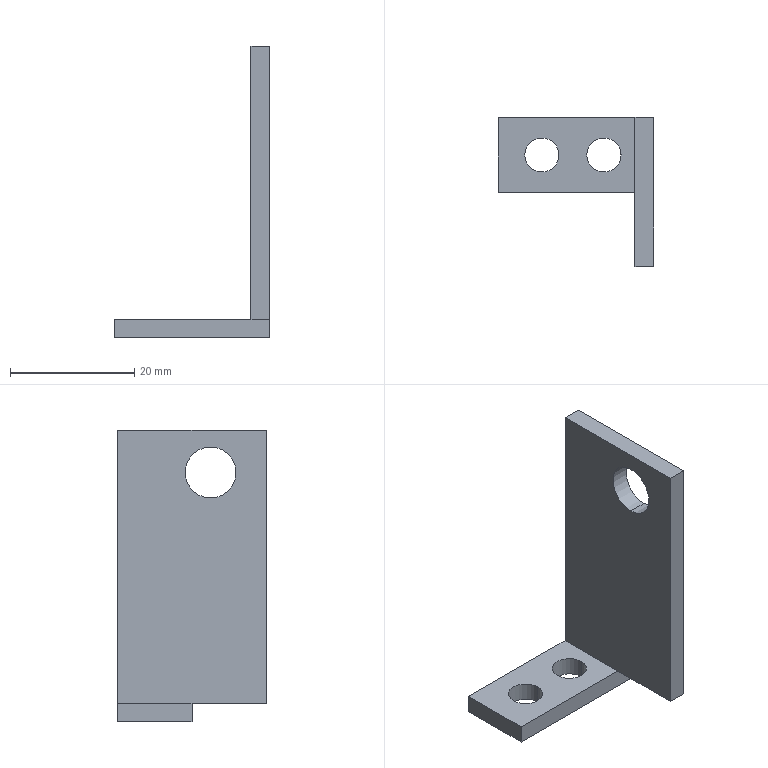Part | 1 solid | 16 faces | box 25 x 24 x 47 mm | volume 3767 mm3 | plane 10 | cylinder 6 | commonest cylinder face diameters 5.5 x4 8.2 x2
STEP:
#1=CARTESIAN_POINT('',(0.,0.,0.));
#2=DIRECTION('',(0.,0.,1.));
#3=DIRECTION('',(1.,0.,0.));
#4=AXIS2_PLACEMENT_3D('',#1,#2,#3);
#5=CARTESIAN_POINT('',(-283.573,419.5,-194.274));
#6=VERTEX_POINT('',#5);
#7=CARTESIAN_POINT('',(-283.573,419.5,-202.474));
#8=VERTEX_POINT('',#7);
#9=CARTESIAN_POINT('',(-283.573,419.5,-198.374));
#10=DIRECTION('',(-1.,0.,0.));
#11=DIRECTION('',(0.,0.,-1.));
#12=AXIS2_PLACEMENT_3D('',#9,#10,#11);
#13=CIRCLE('',#12,4.1);
#14=CARTESIAN_POINT('',(-291.041,419.5,-198.374));
#15=DIRECTION('',(-1.,0.,0.));
#16=DIRECTION('',(0.,-1.,0.));
#17=AXIS2_PLACEMENT_3D('',#14,#15,#16);
#18=CYLINDRICAL_SURFACE('',#17,4.1);
#19=CARTESIAN_POINT('',(-1.571,-7.468));
#20=DIRECTION('',(1.,0.));
#21=VECTOR('',#20,1.);
#22=LINE('',#19,#21);
#23=(GEOMETRIC_REPRESENTATION_CONTEXT(2)PARAMETRIC_REPRESENTATION_CONTEXT()REPRESENTATION_CONTEXT('',''));
#24=DEFINITIONAL_REPRESENTATION('',(#22),#23);
#25=PCURVE('',#18,#24);
#26=CARTESIAN_POINT('',(-283.573,428.525,-194.374));
#27=DIRECTION('',(1.,0.,0.));
#28=DIRECTION('',(0.,-1.,0.));
#29=AXIS2_PLACEMENT_3D('',#26,#27,#28);
#30=PLANE('',#29);
#31=CARTESIAN_POINT('',(9.025,8.1));
#32=CARTESIAN_POINT('',(16.126,8.1));
#33=CARTESIAN_POINT('',(12.576,1.95));
#34=CARTESIAN_POINT('',(9.025,-4.2));
#35=CARTESIAN_POINT('',(5.474,1.95));
#36=CARTESIAN_POINT('',(1.924,8.1));
#37=CARTESIAN_POINT('',(9.025,8.1));
#38=(BOUNDED_CURVE()B_SPLINE_CURVE(2,(#31,#32,#33,#34,#35,#36,#37),.UNSPECIFIED.,.T.,.F.)B_SPLINE_CURVE_WITH_KNOTS((1,2,2,2,2,1),(-2.094,0.,2.094,4.189,6.283,8.378),.UNSPECIFIED.)CURVE()GEOMETRIC_REPRESENTATION_ITEM()RATIONAL_B_SPLINE_CURVE((1.,0.5,1.,0.5,1.,0.5,1.))REPRESENTATION_ITEM(''));
#39=(GEOMETRIC_REPRESENTATION_CONTEXT(2)PARAMETRIC_REPRESENTATION_CONTEXT()REPRESENTATION_CONTEXT('',''));
#40=DEFINITIONAL_REPRESENTATION('',(#38),#39);
#41=PCURVE('',#30,#40);
#42=SURFACE_CURVE('',#13,(#25,#41),.PCURVE_S1.);
#43=EDGE_CURVE('',#6,#8,#42,.T.);
#44=ORIENTED_EDGE('',*,*,#43,.T.);
#45=CARTESIAN_POINT('',(-286.573,419.5,-202.474));
#46=VERTEX_POINT('',#45);
#47=CARTESIAN_POINT('',(-283.573,419.5,-202.474));
#48=DIRECTION('',(-1.,0.,0.));
#49=VECTOR('',#48,1.);
#50=LINE('',#47,#49);
#51=CARTESIAN_POINT('',(4.712,-7.468));
#52=DIRECTION('',(0.,1.));
#53=VECTOR('',#52,1.);
#54=LINE('',#51,#53);
#55=(GEOMETRIC_REPRESENTATION_CONTEXT(2)PARAMETRIC_REPRESENTATION_CONTEXT()REPRESENTATION_CONTEXT('',''));
#56=DEFINITIONAL_REPRESENTATION('',(#54),#55);
#57=PCURVE('',#18,#56);
#58=CARTESIAN_POINT('',(-291.041,419.5,-198.374));
#59=DIRECTION('',(-1.,0.,0.));
#60=DIRECTION('',(0.,1.,0.));
#61=AXIS2_PLACEMENT_3D('',#58,#59,#60);
#62=CYLINDRICAL_SURFACE('',#61,4.1);
#63=CARTESIAN_POINT('',(1.571,-7.468));
#64=DIRECTION('',(0.,1.));
#65=VECTOR('',#64,1.);
#66=LINE('',#63,#65);
#67=(GEOMETRIC_REPRESENTATION_CONTEXT(2)PARAMETRIC_REPRESENTATION_CONTEXT()REPRESENTATION_CONTEXT('',''));
#68=DEFINITIONAL_REPRESENTATION('',(#66),#67);
#69=PCURVE('',#62,#68);
#70=SURFACE_CURVE('',#50,(#57,#69),.PCURVE_S1.);
#71=EDGE_CURVE('',#8,#46,#70,.T.);
#72=ORIENTED_EDGE('',*,*,#71,.T.);
#73=CARTESIAN_POINT('',(-286.573,419.5,-194.274));
#74=VERTEX_POINT('',#73);
#75=CARTESIAN_POINT('',(-286.573,419.5,-198.374));
#76=DIRECTION('',(1.,0.,0.));
#77=DIRECTION('',(0.,0.,-1.));
#78=AXIS2_PLACEMENT_3D('',#75,#76,#77);
#79=CIRCLE('',#78,4.1);
#80=CARTESIAN_POINT('',(4.712,-4.468));
#81=DIRECTION('',(-1.,0.));
#82=VECTOR('',#81,1.);
#83=LINE('',#80,#82);
#84=(GEOMETRIC_REPRESENTATION_CONTEXT(2)PARAMETRIC_REPRESENTATION_CONTEXT()REPRESENTATION_CONTEXT('',''));
#85=DEFINITIONAL_REPRESENTATION('',(#83),#84);
#86=PCURVE('',#18,#85);
#87=CARTESIAN_POINT('',(-286.573,428.525,-194.374));
#88=DIRECTION('',(-1.,0.,0.));
#89=DIRECTION('',(0.,1.,0.));
#90=AXIS2_PLACEMENT_3D('',#87,#88,#89);
#91=PLANE('',#90);
#92=CARTESIAN_POINT('',(-9.025,8.1));
#93=CARTESIAN_POINT('',(-1.924,8.1));
#94=CARTESIAN_POINT('',(-5.474,1.95));
#95=CARTESIAN_POINT('',(-9.025,-4.2));
#96=CARTESIAN_POINT('',(-12.576,1.95));
#97=CARTESIAN_POINT('',(-16.126,8.1));
#98=CARTESIAN_POINT('',(-9.025,8.1));
#99=(BOUNDED_CURVE()B_SPLINE_CURVE(2,(#92,#93,#94,#95,#96,#97,#98),.UNSPECIFIED.,.T.,.F.)B_SPLINE_CURVE_WITH_KNOTS((1,2,2,2,2,1),(-2.094,0.,2.094,4.189,6.283,8.378),.UNSPECIFIED.)CURVE()GEOMETRIC_REPRESENTATION_ITEM()RATIONAL_B_SPLINE_CURVE((1.,0.5,1.,0.5,1.,0.5,1.))REPRESENTATION_ITEM(''));
#100=(GEOMETRIC_REPRESENTATION_CONTEXT(2)PARAMETRIC_REPRESENTATION_CONTEXT()REPRESENTATION_CONTEXT('',''));
#101=DEFINITIONAL_REPRESENTATION('',(#99),#100);
#102=PCURVE('',#91,#101);
#103=SURFACE_CURVE('',#79,(#86,#102),.PCURVE_S1.);
#104=EDGE_CURVE('',#46,#74,#103,.T.);
#105=ORIENTED_EDGE('',*,*,#104,.T.);
#106=CARTESIAN_POINT('',(-283.573,419.5,-194.274));
#107=DIRECTION('',(-1.,0.,0.));
#108=VECTOR('',#107,1.);
#109=LINE('',#106,#108);
#110=CARTESIAN_POINT('',(1.571,-7.468));
#111=DIRECTION('',(0.,1.));
#112=VECTOR('',#111,1.);
#113=LINE('',#110,#112);
#114=(GEOMETRIC_REPRESENTATION_CONTEXT(2)PARAMETRIC_REPRESENTATION_CONTEXT()REPRESENTATION_CONTEXT('',''));
#115=DEFINITIONAL_REPRESENTATION('',(#113),#114);
#116=PCURVE('',#18,#115);
#117=CARTESIAN_POINT('',(4.712,-7.468));
#118=DIRECTION('',(0.,1.));
#119=VECTOR('',#118,1.);
#120=LINE('',#117,#119);
#121=(GEOMETRIC_REPRESENTATION_CONTEXT(2)PARAMETRIC_REPRESENTATION_CONTEXT()REPRESENTATION_CONTEXT('',''));
#122=DEFINITIONAL_REPRESENTATION('',(#120),#121);
#123=PCURVE('',#62,#122);
#124=SURFACE_CURVE('',#109,(#116,#123),.PCURVE_S1.);
#125=EDGE_CURVE('',#6,#74,#124,.T.);
#126=ORIENTED_EDGE('',*,*,#125,.F.);
#127=EDGE_LOOP('',(#44,#72,#105,#126));
#128=FACE_BOUND('',#127,.F.);
#129=ADVANCED_FACE('',(#128),#18,.F.);
#130=CARTESIAN_POINT('',(-286.573,410.5,-191.55));
#131=VERTEX_POINT('',#130);
#132=CARTESIAN_POINT('',(-286.573,434.5,-191.55));
#133=VERTEX_POINT('',#132);
#134=CARTESIAN_POINT('',(-286.573,428.525,-191.55));
#135=DIRECTION('',(0.,1.,0.));
#136=VECTOR('',#135,1.);
#137=LINE('',#134,#136);
#138=CARTESIAN_POINT('',(0.,-2.824));
#139=DIRECTION('',(1.,0.));
#140=VECTOR('',#139,1.);
#141=LINE('',#138,#140);
#142=(GEOMETRIC_REPRESENTATION_CONTEXT(2)PARAMETRIC_REPRESENTATION_CONTEXT()REPRESENTATION_CONTEXT('',''));
#143=DEFINITIONAL_REPRESENTATION('',(#141),#142);
#144=PCURVE('',#91,#143);
#145=CARTESIAN_POINT('',(-153.465,586.5,-191.55));
#146=DIRECTION('',(0.,0.,1.));
#147=DIRECTION('',(-1.,0.,0.));
#148=AXIS2_PLACEMENT_3D('',#145,#146,#147);
#149=PLANE('',#148);
#150=CARTESIAN_POINT('',(133.108,157.975));
#151=DIRECTION('',(0.,-1.));
#152=VECTOR('',#151,1.);
#153=LINE('',#150,#152);
#154=(GEOMETRIC_REPRESENTATION_CONTEXT(2)PARAMETRIC_REPRESENTATION_CONTEXT()REPRESENTATION_CONTEXT('',''));
#155=DEFINITIONAL_REPRESENTATION('',(#153),#154);
#156=PCURVE('',#149,#155);
#157=SURFACE_CURVE('',#137,(#144,#156),.PCURVE_S1.);
#158=EDGE_CURVE('',#131,#133,#157,.T.);
#159=ORIENTED_EDGE('',*,*,#158,.T.);
#160=CARTESIAN_POINT('',(-286.573,434.5,-235.55));
#161=VERTEX_POINT('',#160);
#162=CARTESIAN_POINT('',(-286.573,434.5,-194.374));
#163=DIRECTION('',(0.,0.,1.));
#164=VECTOR('',#163,1.);
#165=LINE('',#162,#164);
#166=CARTESIAN_POINT('',(5.975,0.));
#167=DIRECTION('',(0.,-1.));
#168=VECTOR('',#167,1.);
#169=LINE('',#166,#168);
#170=(GEOMETRIC_REPRESENTATION_CONTEXT(2)PARAMETRIC_REPRESENTATION_CONTEXT()REPRESENTATION_CONTEXT('',''));
#171=DEFINITIONAL_REPRESENTATION('',(#169),#170);
#172=PCURVE('',#91,#171);
#173=CARTESIAN_POINT('',(-285.073,434.5,-194.374));
#174=DIRECTION('',(0.,1.,0.));
#175=DIRECTION('',(1.,0.,0.));
#176=AXIS2_PLACEMENT_3D('',#173,#174,#175);
#177=PLANE('',#176);
#178=CARTESIAN_POINT('',(-1.5,0.));
#179=DIRECTION('',(0.,-1.));
#180=VECTOR('',#179,1.);
#181=LINE('',#178,#180);
#182=(GEOMETRIC_REPRESENTATION_CONTEXT(2)PARAMETRIC_REPRESENTATION_CONTEXT()REPRESENTATION_CONTEXT('',''));
#183=DEFINITIONAL_REPRESENTATION('',(#181),#182);
#184=PCURVE('',#177,#183);
#185=SURFACE_CURVE('',#165,(#172,#184),.PCURVE_S1.);
#186=EDGE_CURVE('',#161,#133,#185,.T.);
#187=ORIENTED_EDGE('',*,*,#186,.F.);
#188=CARTESIAN_POINT('',(-286.573,422.5,-235.55));
#189=VERTEX_POINT('',#188);
#190=CARTESIAN_POINT('',(-286.573,428.525,-235.55));
#191=DIRECTION('',(0.,1.,0.));
#192=VECTOR('',#191,1.);
#193=LINE('',#190,#192);
#194=CARTESIAN_POINT('',(0.,41.176));
#195=DIRECTION('',(1.,0.));
#196=VECTOR('',#195,1.);
#197=LINE('',#194,#196);
#198=(GEOMETRIC_REPRESENTATION_CONTEXT(2)PARAMETRIC_REPRESENTATION_CONTEXT()REPRESENTATION_CONTEXT('',''));
#199=DEFINITIONAL_REPRESENTATION('',(#197),#198);
#200=PCURVE('',#91,#199);
#201=CARTESIAN_POINT('',(-153.465,586.5,-235.55));
#202=DIRECTION('',(0.,0.,1.));
#203=DIRECTION('',(-1.,0.,0.));
#204=AXIS2_PLACEMENT_3D('',#201,#202,#203);
#205=PLANE('',#204);
#206=CARTESIAN_POINT('',(133.108,157.975));
#207=DIRECTION('',(0.,-1.));
#208=VECTOR('',#207,1.);
#209=LINE('',#206,#208);
#210=(GEOMETRIC_REPRESENTATION_CONTEXT(2)PARAMETRIC_REPRESENTATION_CONTEXT()REPRESENTATION_CONTEXT('',''));
#211=DEFINITIONAL_REPRESENTATION('',(#209),#210);
#212=PCURVE('',#205,#211);
#213=SURFACE_CURVE('',#193,(#200,#212),.PCURVE_S1.);
#214=EDGE_CURVE('',#189,#161,#213,.T.);
#215=ORIENTED_EDGE('',*,*,#214,.F.);
#216=CARTESIAN_POINT('',(-286.573,410.5,-235.55));
#217=VERTEX_POINT('',#216);
#218=CARTESIAN_POINT('',(-286.573,428.525,-235.55));
#219=DIRECTION('',(0.,1.,0.));
#220=VECTOR('',#219,1.);
#221=LINE('',#218,#220);
#222=CARTESIAN_POINT('',(0.,41.176));
#223=DIRECTION('',(1.,0.));
#224=VECTOR('',#223,1.);
#225=LINE('',#222,#224);
#226=(GEOMETRIC_REPRESENTATION_CONTEXT(2)PARAMETRIC_REPRESENTATION_CONTEXT()REPRESENTATION_CONTEXT('',''));
#227=DEFINITIONAL_REPRESENTATION('',(#225),#226);
#228=PCURVE('',#91,#227);
#229=CARTESIAN_POINT('',(-295.111,431.125,-235.55));
#230=DIRECTION('',(0.,0.,1.));
#231=DIRECTION('',(-1.,0.,0.));
#232=AXIS2_PLACEMENT_3D('',#229,#230,#231);
#233=PLANE('',#232);
#234=CARTESIAN_POINT('',(-8.537,2.6));
#235=DIRECTION('',(0.,-1.));
#236=VECTOR('',#235,1.);
#237=LINE('',#234,#236);
#238=(GEOMETRIC_REPRESENTATION_CONTEXT(2)PARAMETRIC_REPRESENTATION_CONTEXT()REPRESENTATION_CONTEXT('',''));
#239=DEFINITIONAL_REPRESENTATION('',(#237),#238);
#240=PCURVE('',#233,#239);
#241=SURFACE_CURVE('',#221,(#228,#240),.PCURVE_S1.);
#242=EDGE_CURVE('',#217,#189,#241,.T.);
#243=ORIENTED_EDGE('',*,*,#242,.F.);
#244=CARTESIAN_POINT('',(-286.573,410.5,-67.661));
#245=DIRECTION('',(0.,0.,-1.));
#246=VECTOR('',#245,1.);
#247=LINE('',#244,#246);
#248=CARTESIAN_POINT('',(-18.025,-126.713));
#249=DIRECTION('',(0.,1.));
#250=VECTOR('',#249,1.);
#251=LINE('',#248,#250);
#252=(GEOMETRIC_REPRESENTATION_CONTEXT(2)PARAMETRIC_REPRESENTATION_CONTEXT()REPRESENTATION_CONTEXT('',''));
#253=DEFINITIONAL_REPRESENTATION('',(#251),#252);
#254=PCURVE('',#91,#253);
#255=CARTESIAN_POINT('',(-276.706,410.5,-67.661));
#256=DIRECTION('',(0.,-1.,0.));
#257=DIRECTION('',(1.,0.,0.));
#258=AXIS2_PLACEMENT_3D('',#255,#256,#257);
#259=PLANE('',#258);
#260=CARTESIAN_POINT('',(-9.868,0.));
#261=DIRECTION('',(0.,-1.));
#262=VECTOR('',#261,1.);
#263=LINE('',#260,#262);
#264=(GEOMETRIC_REPRESENTATION_CONTEXT(2)PARAMETRIC_REPRESENTATION_CONTEXT()REPRESENTATION_CONTEXT('',''));
#265=DEFINITIONAL_REPRESENTATION('',(#263),#264);
#266=PCURVE('',#259,#265);
#267=SURFACE_CURVE('',#247,(#254,#266),.PCURVE_S1.);
#268=EDGE_CURVE('',#131,#217,#267,.T.);
#269=ORIENTED_EDGE('',*,*,#268,.F.);
#270=EDGE_LOOP('',(#159,#187,#215,#243,#269));
#271=FACE_BOUND('',#270,.T.);
#272=ORIENTED_EDGE('',*,*,#104,.T.);
#273=CARTESIAN_POINT('',(-286.573,419.5,-198.374));
#274=DIRECTION('',(1.,0.,0.));
#275=DIRECTION('',(0.,0.,-1.));
#276=AXIS2_PLACEMENT_3D('',#273,#274,#275);
#277=CIRCLE('',#276,4.1);
#278=CARTESIAN_POINT('',(-9.025,8.1));
#279=CARTESIAN_POINT('',(-1.924,8.1));
#280=CARTESIAN_POINT('',(-5.474,1.95));
#281=CARTESIAN_POINT('',(-9.025,-4.2));
#282=CARTESIAN_POINT('',(-12.576,1.95));
#283=CARTESIAN_POINT('',(-16.126,8.1));
#284=CARTESIAN_POINT('',(-9.025,8.1));
#285=(BOUNDED_CURVE()B_SPLINE_CURVE(2,(#278,#279,#280,#281,#282,#283,#284),.UNSPECIFIED.,.T.,.F.)B_SPLINE_CURVE_WITH_KNOTS((1,2,2,2,2,1),(-2.094,0.,2.094,4.189,6.283,8.378),.UNSPECIFIED.)CURVE()GEOMETRIC_REPRESENTATION_ITEM()RATIONAL_B_SPLINE_CURVE((1.,0.5,1.,0.5,1.,0.5,1.))REPRESENTATION_ITEM(''));
#286=(GEOMETRIC_REPRESENTATION_CONTEXT(2)PARAMETRIC_REPRESENTATION_CONTEXT()REPRESENTATION_CONTEXT('',''));
#287=DEFINITIONAL_REPRESENTATION('',(#285),#286);
#288=PCURVE('',#91,#287);
#289=CARTESIAN_POINT('',(7.854,-4.468));
#290=DIRECTION('',(-1.,0.));
#291=VECTOR('',#290,1.);
#292=LINE('',#289,#291);
#293=(GEOMETRIC_REPRESENTATION_CONTEXT(2)PARAMETRIC_REPRESENTATION_CONTEXT()REPRESENTATION_CONTEXT('',''));
#294=DEFINITIONAL_REPRESENTATION('',(#292),#293);
#295=PCURVE('',#62,#294);
#296=SURFACE_CURVE('',#277,(#288,#295),.PCURVE_S1.);
#297=EDGE_CURVE('',#74,#46,#296,.T.);
#298=ORIENTED_EDGE('',*,*,#297,.T.);
#299=EDGE_LOOP('',(#272,#298));
#300=FACE_BOUND('',#299,.T.);
#301=ADVANCED_FACE('',(#271,#300),#91,.T.);
#302=CARTESIAN_POINT('',(-283.573,410.5,-235.55));
#303=VERTEX_POINT('',#302);
#304=CARTESIAN_POINT('',(-276.706,410.5,-235.55));
#305=DIRECTION('',(-1.,0.,0.));
#306=VECTOR('',#305,1.);
#307=LINE('',#304,#306);
#308=CARTESIAN_POINT('',(0.,-167.889));
#309=DIRECTION('',(-1.,0.));
#310=VECTOR('',#309,1.);
#311=LINE('',#308,#310);
#312=(GEOMETRIC_REPRESENTATION_CONTEXT(2)PARAMETRIC_REPRESENTATION_CONTEXT()REPRESENTATION_CONTEXT('',''));
#313=DEFINITIONAL_REPRESENTATION('',(#311),#312);
#314=PCURVE('',#259,#313);
#315=CARTESIAN_POINT('',(-18.405,20.625));
#316=DIRECTION('',(1.,0.));
#317=VECTOR('',#316,1.);
#318=LINE('',#315,#317);
#319=(GEOMETRIC_REPRESENTATION_CONTEXT(2)PARAMETRIC_REPRESENTATION_CONTEXT()REPRESENTATION_CONTEXT('',''));
#320=DEFINITIONAL_REPRESENTATION('',(#318),#319);
#321=PCURVE('',#233,#320);
#322=SURFACE_CURVE('',#307,(#314,#321),.PCURVE_S1.);
#323=EDGE_CURVE('',#303,#217,#322,.T.);
#324=ORIENTED_EDGE('',*,*,#323,.F.);
#325=CARTESIAN_POINT('',(-283.573,410.5,-191.55));
#326=VERTEX_POINT('',#325);
#327=CARTESIAN_POINT('',(-283.573,410.5,-67.661));
#328=DIRECTION('',(0.,0.,1.));
#329=VECTOR('',#328,1.);
#330=LINE('',#327,#329);
#331=CARTESIAN_POINT('',(-6.868,0.));
#332=DIRECTION('',(0.,1.));
#333=VECTOR('',#332,1.);
#334=LINE('',#331,#333);
#335=(GEOMETRIC_REPRESENTATION_CONTEXT(2)PARAMETRIC_REPRESENTATION_CONTEXT()REPRESENTATION_CONTEXT('',''));
#336=DEFINITIONAL_REPRESENTATION('',(#334),#335);
#337=PCURVE('',#259,#336);
#338=CARTESIAN_POINT('',(18.025,-126.713));
#339=DIRECTION('',(0.,-1.));
#340=VECTOR('',#339,1.);
#341=LINE('',#338,#340);
#342=(GEOMETRIC_REPRESENTATION_CONTEXT(2)PARAMETRIC_REPRESENTATION_CONTEXT()REPRESENTATION_CONTEXT('',''));
#343=DEFINITIONAL_REPRESENTATION('',(#341),#342);
#344=PCURVE('',#30,#343);
#345=SURFACE_CURVE('',#330,(#337,#344),.PCURVE_S1.);
#346=EDGE_CURVE('',#303,#326,#345,.T.);
#347=ORIENTED_EDGE('',*,*,#346,.T.);
#348=CARTESIAN_POINT('',(-276.706,410.5,-191.55));
#349=DIRECTION('',(-1.,0.,0.));
#350=VECTOR('',#349,1.);
#351=LINE('',#348,#350);
#352=CARTESIAN_POINT('',(0.,-123.889));
#353=DIRECTION('',(-1.,0.));
#354=VECTOR('',#353,1.);
#355=LINE('',#352,#354);
#356=(GEOMETRIC_REPRESENTATION_CONTEXT(2)PARAMETRIC_REPRESENTATION_CONTEXT()REPRESENTATION_CONTEXT('',''));
#357=DEFINITIONAL_REPRESENTATION('',(#355),#356);
#358=PCURVE('',#259,#357);
#359=CARTESIAN_POINT('',(123.24,176.));
#360=DIRECTION('',(1.,0.));
#361=VECTOR('',#360,1.);
#362=LINE('',#359,#361);
#363=(GEOMETRIC_REPRESENTATION_CONTEXT(2)PARAMETRIC_REPRESENTATION_CONTEXT()REPRESENTATION_CONTEXT('',''));
#364=DEFINITIONAL_REPRESENTATION('',(#362),#363);
#365=PCURVE('',#149,#364);
#366=SURFACE_CURVE('',#351,(#358,#365),.PCURVE_S1.);
#367=EDGE_CURVE('',#326,#131,#366,.T.);
#368=ORIENTED_EDGE('',*,*,#367,.T.);
#369=ORIENTED_EDGE('',*,*,#268,.T.);
#370=EDGE_LOOP('',(#324,#347,#368,#369));
#371=FACE_BOUND('',#370,.T.);
#372=ADVANCED_FACE('',(#371),#259,.T.);
#373=CARTESIAN_POINT('',(-283.573,434.5,-191.55));
#374=VERTEX_POINT('',#373);
#375=CARTESIAN_POINT('',(-283.573,586.5,-191.55));
#376=DIRECTION('',(0.,1.,0.));
#377=VECTOR('',#376,1.);
#378=LINE('',#375,#377);
#379=CARTESIAN_POINT('',(130.108,0.));
#380=DIRECTION('',(0.,-1.));
#381=VECTOR('',#380,1.);
#382=LINE('',#379,#381);
#383=(GEOMETRIC_REPRESENTATION_CONTEXT(2)PARAMETRIC_REPRESENTATION_CONTEXT()REPRESENTATION_CONTEXT('',''));
#384=DEFINITIONAL_REPRESENTATION('',(#382),#383);
#385=PCURVE('',#149,#384);
#386=CARTESIAN_POINT('',(-157.975,-2.824));
#387=DIRECTION('',(-1.,0.));
#388=VECTOR('',#387,1.);
#389=LINE('',#386,#388);
#390=(GEOMETRIC_REPRESENTATION_CONTEXT(2)PARAMETRIC_REPRESENTATION_CONTEXT()REPRESENTATION_CONTEXT('',''));
#391=DEFINITIONAL_REPRESENTATION('',(#389),#390);
#392=PCURVE('',#30,#391);
#393=SURFACE_CURVE('',#378,(#385,#392),.PCURVE_S1.);
#394=EDGE_CURVE('',#326,#374,#393,.T.);
#395=ORIENTED_EDGE('',*,*,#394,.T.);
#396=CARTESIAN_POINT('',(-285.073,434.5,-191.55));
#397=DIRECTION('',(1.,0.,0.));
#398=VECTOR('',#397,1.);
#399=LINE('',#396,#398);
#400=CARTESIAN_POINT('',(131.608,152.));
#401=DIRECTION('',(-1.,0.));
#402=VECTOR('',#401,1.);
#403=LINE('',#400,#402);
#404=(GEOMETRIC_REPRESENTATION_CONTEXT(2)PARAMETRIC_REPRESENTATION_CONTEXT()REPRESENTATION_CONTEXT('',''));
#405=DEFINITIONAL_REPRESENTATION('',(#403),#404);
#406=PCURVE('',#149,#405);
#407=CARTESIAN_POINT('',(0.,-2.824));
#408=DIRECTION('',(1.,0.));
#409=VECTOR('',#408,1.);
#410=LINE('',#407,#409);
#411=(GEOMETRIC_REPRESENTATION_CONTEXT(2)PARAMETRIC_REPRESENTATION_CONTEXT()REPRESENTATION_CONTEXT('',''));
#412=DEFINITIONAL_REPRESENTATION('',(#410),#411);
#413=PCURVE('',#177,#412);
#414=SURFACE_CURVE('',#399,(#406,#413),.PCURVE_S1.);
#415=EDGE_CURVE('',#133,#374,#414,.T.);
#416=ORIENTED_EDGE('',*,*,#415,.F.);
#417=ORIENTED_EDGE('',*,*,#158,.F.);
#418=ORIENTED_EDGE('',*,*,#367,.F.);
#419=EDGE_LOOP('',(#395,#416,#417,#418));
#420=FACE_BOUND('',#419,.T.);
#421=ADVANCED_FACE('',(#420),#149,.T.);
#422=CARTESIAN_POINT('',(-283.573,434.5,-238.55));
#423=VERTEX_POINT('',#422);
#424=CARTESIAN_POINT('',(-283.573,434.5,-194.374));
#425=DIRECTION('',(0.,0.,-1.));
#426=VECTOR('',#425,1.);
#427=LINE('',#424,#426);
#428=CARTESIAN_POINT('',(1.5,0.));
#429=DIRECTION('',(0.,1.));
#430=VECTOR('',#429,1.);
#431=LINE('',#428,#430);
#432=(GEOMETRIC_REPRESENTATION_CONTEXT(2)PARAMETRIC_REPRESENTATION_CONTEXT()REPRESENTATION_CONTEXT('',''));
#433=DEFINITIONAL_REPRESENTATION('',(#431),#432);
#434=PCURVE('',#177,#433);
#435=CARTESIAN_POINT('',(-5.975,0.));
#436=DIRECTION('',(0.,1.));
#437=VECTOR('',#436,1.);
#438=LINE('',#435,#437);
#439=(GEOMETRIC_REPRESENTATION_CONTEXT(2)PARAMETRIC_REPRESENTATION_CONTEXT()REPRESENTATION_CONTEXT('',''));
#440=DEFINITIONAL_REPRESENTATION('',(#438),#439);
#441=PCURVE('',#30,#440);
#442=SURFACE_CURVE('',#427,(#434,#441),.PCURVE_S1.);
#443=EDGE_CURVE('',#374,#423,#442,.T.);
#444=ORIENTED_EDGE('',*,*,#443,.T.);
#445=CARTESIAN_POINT('',(-308.573,434.5,-238.55));
#446=VERTEX_POINT('',#445);
#447=CARTESIAN_POINT('',(-285.073,434.5,-238.55));
#448=DIRECTION('',(-1.,0.,0.));
#449=VECTOR('',#448,1.);
#450=LINE('',#447,#449);
#451=CARTESIAN_POINT('',(0.,44.176));
#452=DIRECTION('',(-1.,0.));
#453=VECTOR('',#452,1.);
#454=LINE('',#451,#453);
#455=(GEOMETRIC_REPRESENTATION_CONTEXT(2)PARAMETRIC_REPRESENTATION_CONTEXT()REPRESENTATION_CONTEXT('',''));
#456=DEFINITIONAL_REPRESENTATION('',(#454),#455);
#457=PCURVE('',#177,#456);
#458=CARTESIAN_POINT('',(-153.465,586.5,-238.55));
#459=DIRECTION('',(0.,0.,1.));
#460=DIRECTION('',(-1.,0.,0.));
#461=AXIS2_PLACEMENT_3D('',#458,#459,#460);
#462=PLANE('',#461);
#463=CARTESIAN_POINT('',(131.608,152.));
#464=DIRECTION('',(1.,0.));
#465=VECTOR('',#464,1.);
#466=LINE('',#463,#465);
#467=(GEOMETRIC_REPRESENTATION_CONTEXT(2)PARAMETRIC_REPRESENTATION_CONTEXT()REPRESENTATION_CONTEXT('',''));
#468=DEFINITIONAL_REPRESENTATION('',(#466),#467);
#469=PCURVE('',#462,#468);
#470=SURFACE_CURVE('',#450,(#457,#469),.PCURVE_S1.);
#471=EDGE_CURVE('',#423,#446,#470,.T.);
#472=ORIENTED_EDGE('',*,*,#471,.T.);
#473=CARTESIAN_POINT('',(-308.573,434.5,-235.55));
#474=VERTEX_POINT('',#473);
#475=CARTESIAN_POINT('',(-308.573,434.5,-194.374));
#476=DIRECTION('',(0.,0.,1.));
#477=VECTOR('',#476,1.);
#478=LINE('',#475,#477);
#479=CARTESIAN_POINT('',(-23.5,0.));
#480=DIRECTION('',(0.,-1.));
#481=VECTOR('',#480,1.);
#482=LINE('',#479,#481);
#483=(GEOMETRIC_REPRESENTATION_CONTEXT(2)PARAMETRIC_REPRESENTATION_CONTEXT()REPRESENTATION_CONTEXT('',''));
#484=DEFINITIONAL_REPRESENTATION('',(#482),#483);
#485=PCURVE('',#177,#484);
#486=CARTESIAN_POINT('',(-308.573,428.525,-194.374));
#487=DIRECTION('',(1.,0.,0.));
#488=DIRECTION('',(0.,-1.,0.));
#489=AXIS2_PLACEMENT_3D('',#486,#487,#488);
#490=PLANE('',#489);
#491=CARTESIAN_POINT('',(-5.975,0.));
#492=DIRECTION('',(0.,-1.));
#493=VECTOR('',#492,1.);
#494=LINE('',#491,#493);
#495=(GEOMETRIC_REPRESENTATION_CONTEXT(2)PARAMETRIC_REPRESENTATION_CONTEXT()REPRESENTATION_CONTEXT('',''));
#496=DEFINITIONAL_REPRESENTATION('',(#494),#495);
#497=PCURVE('',#490,#496);
#498=SURFACE_CURVE('',#478,(#485,#497),.PCURVE_S1.);
#499=EDGE_CURVE('',#446,#474,#498,.T.);
#500=ORIENTED_EDGE('',*,*,#499,.T.);
#501=CARTESIAN_POINT('',(-285.073,434.5,-235.55));
#502=DIRECTION('',(1.,0.,0.));
#503=VECTOR('',#502,1.);
#504=LINE('',#501,#503);
#505=CARTESIAN_POINT('',(0.,41.176));
#506=DIRECTION('',(1.,0.));
#507=VECTOR('',#506,1.);
#508=LINE('',#505,#507);
#509=(GEOMETRIC_REPRESENTATION_CONTEXT(2)PARAMETRIC_REPRESENTATION_CONTEXT()REPRESENTATION_CONTEXT('',''));
#510=DEFINITIONAL_REPRESENTATION('',(#508),#509);
#511=PCURVE('',#177,#510);
#512=CARTESIAN_POINT('',(131.608,152.));
#513=DIRECTION('',(-1.,0.));
#514=VECTOR('',#513,1.);
#515=LINE('',#512,#514);
#516=(GEOMETRIC_REPRESENTATION_CONTEXT(2)PARAMETRIC_REPRESENTATION_CONTEXT()REPRESENTATION_CONTEXT('',''));
#517=DEFINITIONAL_REPRESENTATION('',(#515),#516);
#518=PCURVE('',#205,#517);
#519=SURFACE_CURVE('',#504,(#511,#518),.PCURVE_S1.);
#520=EDGE_CURVE('',#474,#161,#519,.T.);
#521=ORIENTED_EDGE('',*,*,#520,.T.);
#522=ORIENTED_EDGE('',*,*,#186,.T.);
#523=ORIENTED_EDGE('',*,*,#415,.T.);
#524=EDGE_LOOP('',(#444,#472,#500,#521,#522,#523));
#525=FACE_BOUND('',#524,.T.);
#526=ADVANCED_FACE('',(#525),#177,.T.);
#527=CARTESIAN_POINT('',(-304.323,428.5,-235.55));
#528=VERTEX_POINT('',#527);
#529=CARTESIAN_POINT('',(-298.823,428.5,-235.55));
#530=VERTEX_POINT('',#529);
#531=CARTESIAN_POINT('',(-301.573,428.5,-235.55));
#532=DIRECTION('',(0.,0.,1.));
#533=DIRECTION('',(1.,0.,0.));
#534=AXIS2_PLACEMENT_3D('',#531,#532,#533);
#535=CIRCLE('',#534,2.75);
#536=CARTESIAN_POINT('',(148.108,158.));
#537=DIRECTION('',(-1.,0.));
#538=AXIS2_PLACEMENT_2D('',#536,#537);
#539=CIRCLE('',#538,2.75);
#540=(GEOMETRIC_REPRESENTATION_CONTEXT(2)PARAMETRIC_REPRESENTATION_CONTEXT()REPRESENTATION_CONTEXT('',''));
#541=DEFINITIONAL_REPRESENTATION('',(#539),#540);
#542=PCURVE('',#205,#541);
#543=CARTESIAN_POINT('',(-301.573,428.5,-235.55));
#544=DIRECTION('',(0.,0.,-1.));
#545=DIRECTION('',(0.,1.,0.));
#546=AXIS2_PLACEMENT_3D('',#543,#544,#545);
#547=CYLINDRICAL_SURFACE('',#546,2.75);
#548=CARTESIAN_POINT('',(7.854,0.));
#549=DIRECTION('',(-1.,0.));
#550=VECTOR('',#549,1.);
#551=LINE('',#548,#550);
#552=(GEOMETRIC_REPRESENTATION_CONTEXT(2)PARAMETRIC_REPRESENTATION_CONTEXT()REPRESENTATION_CONTEXT('',''));
#553=DEFINITIONAL_REPRESENTATION('',(#551),#552);
#554=PCURVE('',#547,#553);
#555=SURFACE_CURVE('',#535,(#542,#554),.PCURVE_S1.);
#556=EDGE_CURVE('',#528,#530,#555,.T.);
#557=ORIENTED_EDGE('',*,*,#556,.F.);
#558=CARTESIAN_POINT('',(-301.573,428.5,-235.55));
#559=DIRECTION('',(0.,0.,1.));
#560=DIRECTION('',(1.,0.,0.));
#561=AXIS2_PLACEMENT_3D('',#558,#559,#560);
#562=CIRCLE('',#561,2.75);
#563=CARTESIAN_POINT('',(148.108,158.));
#564=DIRECTION('',(-1.,0.));
#565=AXIS2_PLACEMENT_2D('',#563,#564);
#566=CIRCLE('',#565,2.75);
#567=(GEOMETRIC_REPRESENTATION_CONTEXT(2)PARAMETRIC_REPRESENTATION_CONTEXT()REPRESENTATION_CONTEXT('',''));
#568=DEFINITIONAL_REPRESENTATION('',(#566),#567);
#569=PCURVE('',#205,#568);
#570=CARTESIAN_POINT('',(-301.573,428.5,-235.55));
#571=DIRECTION('',(0.,0.,-1.));
#572=DIRECTION('',(0.,-1.,0.));
#573=AXIS2_PLACEMENT_3D('',#570,#571,#572);
#574=CYLINDRICAL_SURFACE('',#573,2.75);
#575=CARTESIAN_POINT('',(4.712,0.));
#576=DIRECTION('',(-1.,0.));
#577=VECTOR('',#576,1.);
#578=LINE('',#575,#577);
#579=(GEOMETRIC_REPRESENTATION_CONTEXT(2)PARAMETRIC_REPRESENTATION_CONTEXT()REPRESENTATION_CONTEXT('',''));
#580=DEFINITIONAL_REPRESENTATION('',(#578),#579);
#581=PCURVE('',#574,#580);
#582=SURFACE_CURVE('',#562,(#569,#581),.PCURVE_S1.);
#583=EDGE_CURVE('',#530,#528,#582,.T.);
#584=ORIENTED_EDGE('',*,*,#583,.F.);
#585=EDGE_LOOP('',(#557,#584));
#586=FACE_BOUND('',#585,.T.);
#587=CARTESIAN_POINT('',(-288.823,428.5,-235.55));
#588=VERTEX_POINT('',#587);
#589=CARTESIAN_POINT('',(-294.323,428.5,-235.55));
#590=VERTEX_POINT('',#589);
#591=CARTESIAN_POINT('',(-291.573,428.5,-235.55));
#592=DIRECTION('',(0.,0.,-1.));
#593=DIRECTION('',(1.,0.,0.));
#594=AXIS2_PLACEMENT_3D('',#591,#592,#593);
#595=CIRCLE('',#594,2.75);
#596=CARTESIAN_POINT('',(135.358,158.));
#597=CARTESIAN_POINT('',(135.358,162.763));
#598=CARTESIAN_POINT('',(139.483,160.382));
#599=CARTESIAN_POINT('',(143.608,158.));
#600=CARTESIAN_POINT('',(139.483,155.618));
#601=CARTESIAN_POINT('',(135.358,153.237));
#602=CARTESIAN_POINT('',(135.358,158.));
#603=(BOUNDED_CURVE()B_SPLINE_CURVE(2,(#596,#597,#598,#599,#600,#601,#602),.UNSPECIFIED.,.T.,.F.)B_SPLINE_CURVE_WITH_KNOTS((1,2,2,2,2,1),(-2.094,0.,2.094,4.189,6.283,8.378),.UNSPECIFIED.)CURVE()GEOMETRIC_REPRESENTATION_ITEM()RATIONAL_B_SPLINE_CURVE((1.,0.5,1.,0.5,1.,0.5,1.))REPRESENTATION_ITEM(''));
#604=(GEOMETRIC_REPRESENTATION_CONTEXT(2)PARAMETRIC_REPRESENTATION_CONTEXT()REPRESENTATION_CONTEXT('',''));
#605=DEFINITIONAL_REPRESENTATION('',(#603),#604);
#606=PCURVE('',#205,#605);
#607=CARTESIAN_POINT('',(-291.573,428.5,-235.55));
#608=DIRECTION('',(0.,0.,-1.));
#609=DIRECTION('',(0.,1.,0.));
#610=AXIS2_PLACEMENT_3D('',#607,#608,#609);
#611=CYLINDRICAL_SURFACE('',#610,2.75);
#612=CARTESIAN_POINT('',(1.571,0.));
#613=DIRECTION('',(1.,0.));
#614=VECTOR('',#613,1.);
#615=LINE('',#612,#614);
#616=(GEOMETRIC_REPRESENTATION_CONTEXT(2)PARAMETRIC_REPRESENTATION_CONTEXT()REPRESENTATION_CONTEXT('',''));
#617=DEFINITIONAL_REPRESENTATION('',(#615),#616);
#618=PCURVE('',#611,#617);
#619=SURFACE_CURVE('',#595,(#606,#618),.PCURVE_S1.);
#620=EDGE_CURVE('',#588,#590,#619,.T.);
#621=ORIENTED_EDGE('',*,*,#620,.T.);
#622=CARTESIAN_POINT('',(-291.573,428.5,-235.55));
#623=DIRECTION('',(0.,0.,-1.));
#624=DIRECTION('',(1.,0.,0.));
#625=AXIS2_PLACEMENT_3D('',#622,#623,#624);
#626=CIRCLE('',#625,2.75);
#627=CARTESIAN_POINT('',(135.358,158.));
#628=CARTESIAN_POINT('',(135.358,162.763));
#629=CARTESIAN_POINT('',(139.483,160.382));
#630=CARTESIAN_POINT('',(143.608,158.));
#631=CARTESIAN_POINT('',(139.483,155.618));
#632=CARTESIAN_POINT('',(135.358,153.237));
#633=CARTESIAN_POINT('',(135.358,158.));
#634=(BOUNDED_CURVE()B_SPLINE_CURVE(2,(#627,#628,#629,#630,#631,#632,#633),.UNSPECIFIED.,.T.,.F.)B_SPLINE_CURVE_WITH_KNOTS((1,2,2,2,2,1),(-2.094,0.,2.094,4.189,6.283,8.378),.UNSPECIFIED.)CURVE()GEOMETRIC_REPRESENTATION_ITEM()RATIONAL_B_SPLINE_CURVE((1.,0.5,1.,0.5,1.,0.5,1.))REPRESENTATION_ITEM(''));
#635=(GEOMETRIC_REPRESENTATION_CONTEXT(2)PARAMETRIC_REPRESENTATION_CONTEXT()REPRESENTATION_CONTEXT('',''));
#636=DEFINITIONAL_REPRESENTATION('',(#634),#635);
#637=PCURVE('',#205,#636);
#638=CARTESIAN_POINT('',(-291.573,428.5,-235.55));
#639=DIRECTION('',(0.,0.,-1.));
#640=DIRECTION('',(0.,-1.,0.));
#641=AXIS2_PLACEMENT_3D('',#638,#639,#640);
#642=CYLINDRICAL_SURFACE('',#641,2.75);
#643=CARTESIAN_POINT('',(-1.571,0.));
#644=DIRECTION('',(1.,0.));
#645=VECTOR('',#644,1.);
#646=LINE('',#643,#645);
#647=(GEOMETRIC_REPRESENTATION_CONTEXT(2)PARAMETRIC_REPRESENTATION_CONTEXT()REPRESENTATION_CONTEXT('',''));
#648=DEFINITIONAL_REPRESENTATION('',(#646),#647);
#649=PCURVE('',#642,#648);
#650=SURFACE_CURVE('',#626,(#637,#649),.PCURVE_S1.);
#651=EDGE_CURVE('',#590,#588,#650,.T.);
#652=ORIENTED_EDGE('',*,*,#651,.T.);
#653=EDGE_LOOP('',(#621,#652));
#654=FACE_BOUND('',#653,.T.);
#655=CARTESIAN_POINT('',(-308.573,422.5,-235.55));
#656=VERTEX_POINT('',#655);
#657=CARTESIAN_POINT('',(-276.706,422.5,-235.55));
#658=DIRECTION('',(-1.,0.,0.));
#659=VECTOR('',#658,1.);
#660=LINE('',#657,#659);
#661=CARTESIAN_POINT('',(123.24,164.));
#662=DIRECTION('',(1.,0.));
#663=VECTOR('',#662,1.);
#664=LINE('',#661,#663);
#665=(GEOMETRIC_REPRESENTATION_CONTEXT(2)PARAMETRIC_REPRESENTATION_CONTEXT()REPRESENTATION_CONTEXT('',''));
#666=DEFINITIONAL_REPRESENTATION('',(#664),#665);
#667=PCURVE('',#205,#666);
#668=CARTESIAN_POINT('',(-276.706,422.5,-67.661));
#669=DIRECTION('',(0.,-1.,0.));
#670=DIRECTION('',(1.,0.,0.));
#671=AXIS2_PLACEMENT_3D('',#668,#669,#670);
#672=PLANE('',#671);
#673=CARTESIAN_POINT('',(0.,-167.889));
#674=DIRECTION('',(-1.,0.));
#675=VECTOR('',#674,1.);
#676=LINE('',#673,#675);
#677=(GEOMETRIC_REPRESENTATION_CONTEXT(2)PARAMETRIC_REPRESENTATION_CONTEXT()REPRESENTATION_CONTEXT('',''));
#678=DEFINITIONAL_REPRESENTATION('',(#676),#677);
#679=PCURVE('',#672,#678);
#680=SURFACE_CURVE('',#660,(#667,#679),.PCURVE_S1.);
#681=EDGE_CURVE('',#189,#656,#680,.T.);
#682=ORIENTED_EDGE('',*,*,#681,.F.);
#683=ORIENTED_EDGE('',*,*,#214,.T.);
#684=ORIENTED_EDGE('',*,*,#520,.F.);
#685=CARTESIAN_POINT('',(-308.573,428.525,-235.55));
#686=DIRECTION('',(0.,1.,0.));
#687=VECTOR('',#686,1.);
#688=LINE('',#685,#687);
#689=CARTESIAN_POINT('',(155.108,157.975));
#690=DIRECTION('',(0.,-1.));
#691=VECTOR('',#690,1.);
#692=LINE('',#689,#691);
#693=(GEOMETRIC_REPRESENTATION_CONTEXT(2)PARAMETRIC_REPRESENTATION_CONTEXT()REPRESENTATION_CONTEXT('',''));
#694=DEFINITIONAL_REPRESENTATION('',(#692),#693);
#695=PCURVE('',#205,#694);
#696=CARTESIAN_POINT('',(0.,41.176));
#697=DIRECTION('',(-1.,0.));
#698=VECTOR('',#697,1.);
#699=LINE('',#696,#698);
#700=(GEOMETRIC_REPRESENTATION_CONTEXT(2)PARAMETRIC_REPRESENTATION_CONTEXT()REPRESENTATION_CONTEXT('',''));
#701=DEFINITIONAL_REPRESENTATION('',(#699),#700);
#702=PCURVE('',#490,#701);
#703=SURFACE_CURVE('',#688,(#695,#702),.PCURVE_S1.);
#704=EDGE_CURVE('',#656,#474,#703,.T.);
#705=ORIENTED_EDGE('',*,*,#704,.F.);
#706=EDGE_LOOP('',(#682,#683,#684,#705));
#707=FACE_BOUND('',#706,.T.);
#708=ADVANCED_FACE('',(#586,#654,#707),#205,.T.);
#709=ORIENTED_EDGE('',*,*,#704,.T.);
#710=ORIENTED_EDGE('',*,*,#499,.F.);
#711=CARTESIAN_POINT('',(-308.573,422.5,-238.55));
#712=VERTEX_POINT('',#711);
#713=CARTESIAN_POINT('',(-308.573,586.5,-238.55));
#714=DIRECTION('',(0.,1.,0.));
#715=VECTOR('',#714,1.);
#716=LINE('',#713,#715);
#717=CARTESIAN_POINT('',(-157.975,44.176));
#718=DIRECTION('',(-1.,0.));
#719=VECTOR('',#718,1.);
#720=LINE('',#717,#719);
#721=(GEOMETRIC_REPRESENTATION_CONTEXT(2)PARAMETRIC_REPRESENTATION_CONTEXT()REPRESENTATION_CONTEXT('',''));
#722=DEFINITIONAL_REPRESENTATION('',(#720),#721);
#723=PCURVE('',#490,#722);
#724=CARTESIAN_POINT('',(155.108,0.));
#725=DIRECTION('',(0.,-1.));
#726=VECTOR('',#725,1.);
#727=LINE('',#724,#726);
#728=(GEOMETRIC_REPRESENTATION_CONTEXT(2)PARAMETRIC_REPRESENTATION_CONTEXT()REPRESENTATION_CONTEXT('',''));
#729=DEFINITIONAL_REPRESENTATION('',(#727),#728);
#730=PCURVE('',#462,#729);
#731=SURFACE_CURVE('',#716,(#723,#730),.PCURVE_S1.);
#732=EDGE_CURVE('',#712,#446,#731,.T.);
#733=ORIENTED_EDGE('',*,*,#732,.F.);
#734=CARTESIAN_POINT('',(-308.573,422.5,-67.661));
#735=DIRECTION('',(0.,0.,-1.));
#736=VECTOR('',#735,1.);
#737=LINE('',#734,#736);
#738=CARTESIAN_POINT('',(6.025,-126.713));
#739=DIRECTION('',(0.,1.));
#740=VECTOR('',#739,1.);
#741=LINE('',#738,#740);
#742=(GEOMETRIC_REPRESENTATION_CONTEXT(2)PARAMETRIC_REPRESENTATION_CONTEXT()REPRESENTATION_CONTEXT('',''));
#743=DEFINITIONAL_REPRESENTATION('',(#741),#742);
#744=PCURVE('',#490,#743);
#745=CARTESIAN_POINT('',(-31.868,0.));
#746=DIRECTION('',(0.,-1.));
#747=VECTOR('',#746,1.);
#748=LINE('',#745,#747);
#749=(GEOMETRIC_REPRESENTATION_CONTEXT(2)PARAMETRIC_REPRESENTATION_CONTEXT()REPRESENTATION_CONTEXT('',''));
#750=DEFINITIONAL_REPRESENTATION('',(#748),#749);
#751=PCURVE('',#672,#750);
#752=SURFACE_CURVE('',#737,(#744,#751),.PCURVE_S1.);
#753=EDGE_CURVE('',#656,#712,#752,.T.);
#754=ORIENTED_EDGE('',*,*,#753,.F.);
#755=EDGE_LOOP('',(#709,#710,#733,#754));
#756=FACE_BOUND('',#755,.T.);
#757=ADVANCED_FACE('',(#756),#490,.F.);
#758=CARTESIAN_POINT('',(-283.573,422.5,-238.55));
#759=VERTEX_POINT('',#758);
#760=CARTESIAN_POINT('',(-283.573,422.5,-235.55));
#761=VERTEX_POINT('',#760);
#762=CARTESIAN_POINT('',(-283.573,422.5,-67.661));
#763=DIRECTION('',(0.,0.,1.));
#764=VECTOR('',#763,1.);
#765=LINE('',#762,#764);
#766=CARTESIAN_POINT('',(-6.868,0.));
#767=DIRECTION('',(0.,1.));
#768=VECTOR('',#767,1.);
#769=LINE('',#766,#768);
#770=(GEOMETRIC_REPRESENTATION_CONTEXT(2)PARAMETRIC_REPRESENTATION_CONTEXT()REPRESENTATION_CONTEXT('',''));
#771=DEFINITIONAL_REPRESENTATION('',(#769),#770);
#772=PCURVE('',#672,#771);
#773=CARTESIAN_POINT('',(6.025,-126.713));
#774=DIRECTION('',(0.,-1.));
#775=VECTOR('',#774,1.);
#776=LINE('',#773,#775);
#777=(GEOMETRIC_REPRESENTATION_CONTEXT(2)PARAMETRIC_REPRESENTATION_CONTEXT()REPRESENTATION_CONTEXT('',''));
#778=DEFINITIONAL_REPRESENTATION('',(#776),#777);
#779=PCURVE('',#30,#778);
#780=SURFACE_CURVE('',#765,(#772,#779),.PCURVE_S1.);
#781=EDGE_CURVE('',#759,#761,#780,.T.);
#782=ORIENTED_EDGE('',*,*,#781,.T.);
#783=CARTESIAN_POINT('',(-276.706,422.5,-235.55));
#784=DIRECTION('',(-1.,0.,0.));
#785=VECTOR('',#784,1.);
#786=LINE('',#783,#785);
#787=CARTESIAN_POINT('',(0.,-167.889));
#788=DIRECTION('',(-1.,0.));
#789=VECTOR('',#788,1.);
#790=LINE('',#787,#789);
#791=(GEOMETRIC_REPRESENTATION_CONTEXT(2)PARAMETRIC_REPRESENTATION_CONTEXT()REPRESENTATION_CONTEXT('',''));
#792=DEFINITIONAL_REPRESENTATION('',(#790),#791);
#793=PCURVE('',#672,#792);
#794=CARTESIAN_POINT('',(-18.405,8.625));
#795=DIRECTION('',(1.,0.));
#796=VECTOR('',#795,1.);
#797=LINE('',#794,#796);
#798=(GEOMETRIC_REPRESENTATION_CONTEXT(2)PARAMETRIC_REPRESENTATION_CONTEXT()REPRESENTATION_CONTEXT('',''));
#799=DEFINITIONAL_REPRESENTATION('',(#797),#798);
#800=PCURVE('',#233,#799);
#801=SURFACE_CURVE('',#786,(#793,#800),.PCURVE_S1.);
#802=EDGE_CURVE('',#761,#189,#801,.T.);
#803=ORIENTED_EDGE('',*,*,#802,.T.);
#804=ORIENTED_EDGE('',*,*,#681,.T.);
#805=ORIENTED_EDGE('',*,*,#753,.T.);
#806=CARTESIAN_POINT('',(-276.706,422.5,-238.55));
#807=DIRECTION('',(1.,0.,0.));
#808=VECTOR('',#807,1.);
#809=LINE('',#806,#808);
#810=CARTESIAN_POINT('',(0.,-170.889));
#811=DIRECTION('',(1.,0.));
#812=VECTOR('',#811,1.);
#813=LINE('',#810,#812);
#814=(GEOMETRIC_REPRESENTATION_CONTEXT(2)PARAMETRIC_REPRESENTATION_CONTEXT()REPRESENTATION_CONTEXT('',''));
#815=DEFINITIONAL_REPRESENTATION('',(#813),#814);
#816=PCURVE('',#672,#815);
#817=CARTESIAN_POINT('',(123.24,164.));
#818=DIRECTION('',(-1.,0.));
#819=VECTOR('',#818,1.);
#820=LINE('',#817,#819);
#821=(GEOMETRIC_REPRESENTATION_CONTEXT(2)PARAMETRIC_REPRESENTATION_CONTEXT()REPRESENTATION_CONTEXT('',''));
#822=DEFINITIONAL_REPRESENTATION('',(#820),#821);
#823=PCURVE('',#462,#822);
#824=SURFACE_CURVE('',#809,(#816,#823),.PCURVE_S1.);
#825=EDGE_CURVE('',#712,#759,#824,.T.);
#826=ORIENTED_EDGE('',*,*,#825,.T.);
#827=EDGE_LOOP('',(#782,#803,#804,#805,#826));
#828=FACE_BOUND('',#827,.T.);
#829=ADVANCED_FACE('',(#828),#672,.T.);
#830=CARTESIAN_POINT('',(-304.323,428.5,-238.55));
#831=VERTEX_POINT('',#830);
#832=CARTESIAN_POINT('',(-298.823,428.5,-238.55));
#833=VERTEX_POINT('',#832);
#834=CARTESIAN_POINT('',(-301.573,428.5,-238.55));
#835=DIRECTION('',(0.,0.,-1.));
#836=DIRECTION('',(1.,0.,0.));
#837=AXIS2_PLACEMENT_3D('',#834,#835,#836);
#838=CIRCLE('',#837,2.75);
#839=CARTESIAN_POINT('',(145.358,158.));
#840=CARTESIAN_POINT('',(145.358,162.763));
#841=CARTESIAN_POINT('',(149.483,160.382));
#842=CARTESIAN_POINT('',(153.608,158.));
#843=CARTESIAN_POINT('',(149.483,155.618));
#844=CARTESIAN_POINT('',(145.358,153.237));
#845=CARTESIAN_POINT('',(145.358,158.));
#846=(BOUNDED_CURVE()B_SPLINE_CURVE(2,(#839,#840,#841,#842,#843,#844,#845),.UNSPECIFIED.,.T.,.F.)B_SPLINE_CURVE_WITH_KNOTS((1,2,2,2,2,1),(-2.094,0.,2.094,4.189,6.283,8.378),.UNSPECIFIED.)CURVE()GEOMETRIC_REPRESENTATION_ITEM()RATIONAL_B_SPLINE_CURVE((1.,0.5,1.,0.5,1.,0.5,1.))REPRESENTATION_ITEM(''));
#847=(GEOMETRIC_REPRESENTATION_CONTEXT(2)PARAMETRIC_REPRESENTATION_CONTEXT()REPRESENTATION_CONTEXT('',''));
#848=DEFINITIONAL_REPRESENTATION('',(#846),#847);
#849=PCURVE('',#462,#848);
#850=CARTESIAN_POINT('',(-1.571,3.));
#851=DIRECTION('',(1.,0.));
#852=VECTOR('',#851,1.);
#853=LINE('',#850,#852);
#854=(GEOMETRIC_REPRESENTATION_CONTEXT(2)PARAMETRIC_REPRESENTATION_CONTEXT()REPRESENTATION_CONTEXT('',''));
#855=DEFINITIONAL_REPRESENTATION('',(#853),#854);
#856=PCURVE('',#574,#855);
#857=SURFACE_CURVE('',#838,(#849,#856),.PCURVE_S1.);
#858=EDGE_CURVE('',#831,#833,#857,.T.);
#859=ORIENTED_EDGE('',*,*,#858,.F.);
#860=CARTESIAN_POINT('',(-301.573,428.5,-238.55));
#861=DIRECTION('',(0.,0.,-1.));
#862=DIRECTION('',(1.,0.,0.));
#863=AXIS2_PLACEMENT_3D('',#860,#861,#862);
#864=CIRCLE('',#863,2.75);
#865=CARTESIAN_POINT('',(145.358,158.));
#866=CARTESIAN_POINT('',(145.358,162.763));
#867=CARTESIAN_POINT('',(149.483,160.382));
#868=CARTESIAN_POINT('',(153.608,158.));
#869=CARTESIAN_POINT('',(149.483,155.618));
#870=CARTESIAN_POINT('',(145.358,153.237));
#871=CARTESIAN_POINT('',(145.358,158.));
#872=(BOUNDED_CURVE()B_SPLINE_CURVE(2,(#865,#866,#867,#868,#869,#870,#871),.UNSPECIFIED.,.T.,.F.)B_SPLINE_CURVE_WITH_KNOTS((1,2,2,2,2,1),(-2.094,0.,2.094,4.189,6.283,8.378),.UNSPECIFIED.)CURVE()GEOMETRIC_REPRESENTATION_ITEM()RATIONAL_B_SPLINE_CURVE((1.,0.5,1.,0.5,1.,0.5,1.))REPRESENTATION_ITEM(''));
#873=(GEOMETRIC_REPRESENTATION_CONTEXT(2)PARAMETRIC_REPRESENTATION_CONTEXT()REPRESENTATION_CONTEXT('',''));
#874=DEFINITIONAL_REPRESENTATION('',(#872),#873);
#875=PCURVE('',#462,#874);
#876=CARTESIAN_POINT('',(1.571,3.));
#877=DIRECTION('',(1.,0.));
#878=VECTOR('',#877,1.);
#879=LINE('',#876,#878);
#880=(GEOMETRIC_REPRESENTATION_CONTEXT(2)PARAMETRIC_REPRESENTATION_CONTEXT()REPRESENTATION_CONTEXT('',''));
#881=DEFINITIONAL_REPRESENTATION('',(#879),#880);
#882=PCURVE('',#547,#881);
#883=SURFACE_CURVE('',#864,(#875,#882),.PCURVE_S1.);
#884=EDGE_CURVE('',#833,#831,#883,.T.);
#885=ORIENTED_EDGE('',*,*,#884,.F.);
#886=EDGE_LOOP('',(#859,#885));
#887=FACE_BOUND('',#886,.T.);
#888=CARTESIAN_POINT('',(-294.323,428.5,-238.55));
#889=VERTEX_POINT('',#888);
#890=CARTESIAN_POINT('',(-288.823,428.5,-238.55));
#891=VERTEX_POINT('',#890);
#892=CARTESIAN_POINT('',(-291.573,428.5,-238.55));
#893=DIRECTION('',(0.,0.,-1.));
#894=DIRECTION('',(1.,0.,0.));
#895=AXIS2_PLACEMENT_3D('',#892,#893,#894);
#896=CIRCLE('',#895,2.75);
#897=CARTESIAN_POINT('',(135.358,158.));
#898=CARTESIAN_POINT('',(135.358,162.763));
#899=CARTESIAN_POINT('',(139.483,160.382));
#900=CARTESIAN_POINT('',(143.608,158.));
#901=CARTESIAN_POINT('',(139.483,155.618));
#902=CARTESIAN_POINT('',(135.358,153.237));
#903=CARTESIAN_POINT('',(135.358,158.));
#904=(BOUNDED_CURVE()B_SPLINE_CURVE(2,(#897,#898,#899,#900,#901,#902,#903),.UNSPECIFIED.,.T.,.F.)B_SPLINE_CURVE_WITH_KNOTS((1,2,2,2,2,1),(-2.094,0.,2.094,4.189,6.283,8.378),.UNSPECIFIED.)CURVE()GEOMETRIC_REPRESENTATION_ITEM()RATIONAL_B_SPLINE_CURVE((1.,0.5,1.,0.5,1.,0.5,1.))REPRESENTATION_ITEM(''));
#905=(GEOMETRIC_REPRESENTATION_CONTEXT(2)PARAMETRIC_REPRESENTATION_CONTEXT()REPRESENTATION_CONTEXT('',''));
#906=DEFINITIONAL_REPRESENTATION('',(#904),#905);
#907=PCURVE('',#462,#906);
#908=CARTESIAN_POINT('',(-1.571,3.));
#909=DIRECTION('',(1.,0.));
#910=VECTOR('',#909,1.);
#911=LINE('',#908,#910);
#912=(GEOMETRIC_REPRESENTATION_CONTEXT(2)PARAMETRIC_REPRESENTATION_CONTEXT()REPRESENTATION_CONTEXT('',''));
#913=DEFINITIONAL_REPRESENTATION('',(#911),#912);
#914=PCURVE('',#642,#913);
#915=SURFACE_CURVE('',#896,(#907,#914),.PCURVE_S1.);
#916=EDGE_CURVE('',#889,#891,#915,.T.);
#917=ORIENTED_EDGE('',*,*,#916,.F.);
#918=CARTESIAN_POINT('',(-291.573,428.5,-238.55));
#919=DIRECTION('',(0.,0.,-1.));
#920=DIRECTION('',(1.,0.,0.));
#921=AXIS2_PLACEMENT_3D('',#918,#919,#920);
#922=CIRCLE('',#921,2.75);
#923=CARTESIAN_POINT('',(135.358,158.));
#924=CARTESIAN_POINT('',(135.358,162.763));
#925=CARTESIAN_POINT('',(139.483,160.382));
#926=CARTESIAN_POINT('',(143.608,158.));
#927=CARTESIAN_POINT('',(139.483,155.618));
#928=CARTESIAN_POINT('',(135.358,153.237));
#929=CARTESIAN_POINT('',(135.358,158.));
#930=(BOUNDED_CURVE()B_SPLINE_CURVE(2,(#923,#924,#925,#926,#927,#928,#929),.UNSPECIFIED.,.T.,.F.)B_SPLINE_CURVE_WITH_KNOTS((1,2,2,2,2,1),(-2.094,0.,2.094,4.189,6.283,8.378),.UNSPECIFIED.)CURVE()GEOMETRIC_REPRESENTATION_ITEM()RATIONAL_B_SPLINE_CURVE((1.,0.5,1.,0.5,1.,0.5,1.))REPRESENTATION_ITEM(''));
#931=(GEOMETRIC_REPRESENTATION_CONTEXT(2)PARAMETRIC_REPRESENTATION_CONTEXT()REPRESENTATION_CONTEXT('',''));
#932=DEFINITIONAL_REPRESENTATION('',(#930),#931);
#933=PCURVE('',#462,#932);
#934=CARTESIAN_POINT('',(1.571,3.));
#935=DIRECTION('',(1.,0.));
#936=VECTOR('',#935,1.);
#937=LINE('',#934,#936);
#938=(GEOMETRIC_REPRESENTATION_CONTEXT(2)PARAMETRIC_REPRESENTATION_CONTEXT()REPRESENTATION_CONTEXT('',''));
#939=DEFINITIONAL_REPRESENTATION('',(#937),#938);
#940=PCURVE('',#611,#939);
#941=SURFACE_CURVE('',#922,(#933,#940),.PCURVE_S1.);
#942=EDGE_CURVE('',#891,#889,#941,.T.);
#943=ORIENTED_EDGE('',*,*,#942,.F.);
#944=EDGE_LOOP('',(#917,#943));
#945=FACE_BOUND('',#944,.T.);
#946=ORIENTED_EDGE('',*,*,#732,.T.);
#947=ORIENTED_EDGE('',*,*,#471,.F.);
#948=CARTESIAN_POINT('',(-283.573,428.525,-238.55));
#949=DIRECTION('',(0.,1.,0.));
#950=VECTOR('',#949,1.);
#951=LINE('',#948,#950);
#952=CARTESIAN_POINT('',(130.108,157.975));
#953=DIRECTION('',(0.,-1.));
#954=VECTOR('',#953,1.);
#955=LINE('',#952,#954);
#956=(GEOMETRIC_REPRESENTATION_CONTEXT(2)PARAMETRIC_REPRESENTATION_CONTEXT()REPRESENTATION_CONTEXT('',''));
#957=DEFINITIONAL_REPRESENTATION('',(#955),#956);
#958=PCURVE('',#462,#957);
#959=CARTESIAN_POINT('',(0.,44.176));
#960=DIRECTION('',(-1.,0.));
#961=VECTOR('',#960,1.);
#962=LINE('',#959,#961);
#963=(GEOMETRIC_REPRESENTATION_CONTEXT(2)PARAMETRIC_REPRESENTATION_CONTEXT()REPRESENTATION_CONTEXT('',''));
#964=DEFINITIONAL_REPRESENTATION('',(#962),#963);
#965=PCURVE('',#30,#964);
#966=SURFACE_CURVE('',#951,(#958,#965),.PCURVE_S1.);
#967=EDGE_CURVE('',#759,#423,#966,.T.);
#968=ORIENTED_EDGE('',*,*,#967,.F.);
#969=ORIENTED_EDGE('',*,*,#825,.F.);
#970=EDGE_LOOP('',(#946,#947,#968,#969));
#971=FACE_BOUND('',#970,.T.);
#972=ADVANCED_FACE('',(#887,#945,#971),#462,.F.);
#973=CARTESIAN_POINT('',(-283.573,428.525,-235.55));
#974=DIRECTION('',(0.,-1.,0.));
#975=VECTOR('',#974,1.);
#976=LINE('',#973,#975);
#977=CARTESIAN_POINT('',(0.,41.176));
#978=DIRECTION('',(1.,0.));
#979=VECTOR('',#978,1.);
#980=LINE('',#977,#979);
#981=(GEOMETRIC_REPRESENTATION_CONTEXT(2)PARAMETRIC_REPRESENTATION_CONTEXT()REPRESENTATION_CONTEXT('',''));
#982=DEFINITIONAL_REPRESENTATION('',(#980),#981);
#983=PCURVE('',#30,#982);
#984=CARTESIAN_POINT('',(-11.537,2.6));
#985=DIRECTION('',(0.,1.));
#986=VECTOR('',#985,1.);
#987=LINE('',#984,#986);
#988=(GEOMETRIC_REPRESENTATION_CONTEXT(2)PARAMETRIC_REPRESENTATION_CONTEXT()REPRESENTATION_CONTEXT('',''));
#989=DEFINITIONAL_REPRESENTATION('',(#987),#988);
#990=PCURVE('',#233,#989);
#991=SURFACE_CURVE('',#976,(#983,#990),.PCURVE_S1.);
#992=EDGE_CURVE('',#761,#303,#991,.T.);
#993=ORIENTED_EDGE('',*,*,#992,.F.);
#994=ORIENTED_EDGE('',*,*,#781,.F.);
#995=ORIENTED_EDGE('',*,*,#967,.T.);
#996=ORIENTED_EDGE('',*,*,#443,.F.);
#997=ORIENTED_EDGE('',*,*,#394,.F.);
#998=ORIENTED_EDGE('',*,*,#346,.F.);
#999=EDGE_LOOP('',(#993,#994,#995,#996,#997,#998));
#1000=FACE_BOUND('',#999,.T.);
#1001=CARTESIAN_POINT('',(-283.573,419.5,-198.374));
#1002=DIRECTION('',(-1.,0.,0.));
#1003=DIRECTION('',(0.,0.,-1.));
#1004=AXIS2_PLACEMENT_3D('',#1001,#1002,#1003);
#1005=CIRCLE('',#1004,4.1);
#1006=CARTESIAN_POINT('',(9.025,8.1));
#1007=CARTESIAN_POINT('',(16.126,8.1));
#1008=CARTESIAN_POINT('',(12.576,1.95));
#1009=CARTESIAN_POINT('',(9.025,-4.2));
#1010=CARTESIAN_POINT('',(5.474,1.95));
#1011=CARTESIAN_POINT('',(1.924,8.1));
#1012=CARTESIAN_POINT('',(9.025,8.1));
#1013=(BOUNDED_CURVE()B_SPLINE_CURVE(2,(#1006,#1007,#1008,#1009,#1010,#1011,#1012),.UNSPECIFIED.,.T.,.F.)B_SPLINE_CURVE_WITH_KNOTS((1,2,2,2,2,1),(-2.094,0.,2.094,4.189,6.283,8.378),.UNSPECIFIED.)CURVE()GEOMETRIC_REPRESENTATION_ITEM()RATIONAL_B_SPLINE_CURVE((1.,0.5,1.,0.5,1.,0.5,1.))REPRESENTATION_ITEM(''));
#1014=(GEOMETRIC_REPRESENTATION_CONTEXT(2)PARAMETRIC_REPRESENTATION_CONTEXT()REPRESENTATION_CONTEXT('',''));
#1015=DEFINITIONAL_REPRESENTATION('',(#1013),#1014);
#1016=PCURVE('',#30,#1015);
#1017=CARTESIAN_POINT('',(1.571,-7.468));
#1018=DIRECTION('',(1.,0.));
#1019=VECTOR('',#1018,1.);
#1020=LINE('',#1017,#1019);
#1021=(GEOMETRIC_REPRESENTATION_CONTEXT(2)PARAMETRIC_REPRESENTATION_CONTEXT()REPRESENTATION_CONTEXT('',''));
#1022=DEFINITIONAL_REPRESENTATION('',(#1020),#1021);
#1023=PCURVE('',#62,#1022);
#1024=SURFACE_CURVE('',#1005,(#1016,#1023),.PCURVE_S1.);
#1025=EDGE_CURVE('',#8,#6,#1024,.T.);
#1026=ORIENTED_EDGE('',*,*,#1025,.T.);
#1027=ORIENTED_EDGE('',*,*,#43,.T.);
#1028=EDGE_LOOP('',(#1026,#1027));
#1029=FACE_BOUND('',#1028,.T.);
#1030=ADVANCED_FACE('',(#1000,#1029),#30,.T.);
#1031=ORIENTED_EDGE('',*,*,#802,.F.);
#1032=ORIENTED_EDGE('',*,*,#992,.T.);
#1033=ORIENTED_EDGE('',*,*,#323,.T.);
#1034=ORIENTED_EDGE('',*,*,#242,.T.);
#1035=EDGE_LOOP('',(#1031,#1032,#1033,#1034));
#1036=FACE_BOUND('',#1035,.T.);
#1037=ADVANCED_FACE('',(#1036),#233,.F.);
#1038=ORIENTED_EDGE('',*,*,#651,.T.);
#1039=CARTESIAN_POINT('',(-288.823,428.5,-235.55));
#1040=DIRECTION('',(0.,0.,-1.));
#1041=VECTOR('',#1040,1.);
#1042=LINE('',#1039,#1041);
#1043=CARTESIAN_POINT('',(4.712,0.));
#1044=DIRECTION('',(0.,1.));
#1045=VECTOR('',#1044,1.);
#1046=LINE('',#1043,#1045);
#1047=(GEOMETRIC_REPRESENTATION_CONTEXT(2)PARAMETRIC_REPRESENTATION_CONTEXT()REPRESENTATION_CONTEXT('',''));
#1048=DEFINITIONAL_REPRESENTATION('',(#1046),#1047);
#1049=PCURVE('',#642,#1048);
#1050=CARTESIAN_POINT('',(1.571,0.));
#1051=DIRECTION('',(0.,1.));
#1052=VECTOR('',#1051,1.);
#1053=LINE('',#1050,#1052);
#1054=(GEOMETRIC_REPRESENTATION_CONTEXT(2)PARAMETRIC_REPRESENTATION_CONTEXT()REPRESENTATION_CONTEXT('',''));
#1055=DEFINITIONAL_REPRESENTATION('',(#1053),#1054);
#1056=PCURVE('',#611,#1055);
#1057=SURFACE_CURVE('',#1042,(#1049,#1056),.PCURVE_S1.);
#1058=EDGE_CURVE('',#588,#891,#1057,.T.);
#1059=ORIENTED_EDGE('',*,*,#1058,.T.);
#1060=ORIENTED_EDGE('',*,*,#916,.F.);
#1061=CARTESIAN_POINT('',(-294.323,428.5,-235.55));
#1062=DIRECTION('',(0.,0.,-1.));
#1063=VECTOR('',#1062,1.);
#1064=LINE('',#1061,#1063);
#1065=CARTESIAN_POINT('',(1.571,0.));
#1066=DIRECTION('',(0.,1.));
#1067=VECTOR('',#1066,1.);
#1068=LINE('',#1065,#1067);
#1069=(GEOMETRIC_REPRESENTATION_CONTEXT(2)PARAMETRIC_REPRESENTATION_CONTEXT()REPRESENTATION_CONTEXT('',''));
#1070=DEFINITIONAL_REPRESENTATION('',(#1068),#1069);
#1071=PCURVE('',#642,#1070);
#1072=CARTESIAN_POINT('',(4.712,0.));
#1073=DIRECTION('',(0.,1.));
#1074=VECTOR('',#1073,1.);
#1075=LINE('',#1072,#1074);
#1076=(GEOMETRIC_REPRESENTATION_CONTEXT(2)PARAMETRIC_REPRESENTATION_CONTEXT()REPRESENTATION_CONTEXT('',''));
#1077=DEFINITIONAL_REPRESENTATION('',(#1075),#1076);
#1078=PCURVE('',#611,#1077);
#1079=SURFACE_CURVE('',#1064,(#1071,#1078),.PCURVE_S1.);
#1080=EDGE_CURVE('',#590,#889,#1079,.T.);
#1081=ORIENTED_EDGE('',*,*,#1080,.F.);
#1082=EDGE_LOOP('',(#1038,#1059,#1060,#1081));
#1083=FACE_BOUND('',#1082,.F.);
#1084=ADVANCED_FACE('',(#1083),#642,.F.);
#1085=ORIENTED_EDGE('',*,*,#583,.F.);
#1086=CARTESIAN_POINT('',(-298.823,428.5,-235.55));
#1087=DIRECTION('',(0.,0.,-1.));
#1088=VECTOR('',#1087,1.);
#1089=LINE('',#1086,#1088);
#1090=CARTESIAN_POINT('',(4.712,0.));
#1091=DIRECTION('',(0.,1.));
#1092=VECTOR('',#1091,1.);
#1093=LINE('',#1090,#1092);
#1094=(GEOMETRIC_REPRESENTATION_CONTEXT(2)PARAMETRIC_REPRESENTATION_CONTEXT()REPRESENTATION_CONTEXT('',''));
#1095=DEFINITIONAL_REPRESENTATION('',(#1093),#1094);
#1096=PCURVE('',#574,#1095);
#1097=CARTESIAN_POINT('',(1.571,0.));
#1098=DIRECTION('',(0.,1.));
#1099=VECTOR('',#1098,1.);
#1100=LINE('',#1097,#1099);
#1101=(GEOMETRIC_REPRESENTATION_CONTEXT(2)PARAMETRIC_REPRESENTATION_CONTEXT()REPRESENTATION_CONTEXT('',''));
#1102=DEFINITIONAL_REPRESENTATION('',(#1100),#1101);
#1103=PCURVE('',#547,#1102);
#1104=SURFACE_CURVE('',#1089,(#1096,#1103),.PCURVE_S1.);
#1105=EDGE_CURVE('',#530,#833,#1104,.T.);
#1106=ORIENTED_EDGE('',*,*,#1105,.T.);
#1107=ORIENTED_EDGE('',*,*,#858,.F.);
#1108=CARTESIAN_POINT('',(-304.323,428.5,-235.55));
#1109=DIRECTION('',(0.,0.,-1.));
#1110=VECTOR('',#1109,1.);
#1111=LINE('',#1108,#1110);
#1112=CARTESIAN_POINT('',(1.571,0.));
#1113=DIRECTION('',(0.,1.));
#1114=VECTOR('',#1113,1.);
#1115=LINE('',#1112,#1114);
#1116=(GEOMETRIC_REPRESENTATION_CONTEXT(2)PARAMETRIC_REPRESENTATION_CONTEXT()REPRESENTATION_CONTEXT('',''));
#1117=DEFINITIONAL_REPRESENTATION('',(#1115),#1116);
#1118=PCURVE('',#574,#1117);
#1119=CARTESIAN_POINT('',(4.712,0.));
#1120=DIRECTION('',(0.,1.));
#1121=VECTOR('',#1120,1.);
#1122=LINE('',#1119,#1121);
#1123=(GEOMETRIC_REPRESENTATION_CONTEXT(2)PARAMETRIC_REPRESENTATION_CONTEXT()REPRESENTATION_CONTEXT('',''));
#1124=DEFINITIONAL_REPRESENTATION('',(#1122),#1123);
#1125=PCURVE('',#547,#1124);
#1126=SURFACE_CURVE('',#1111,(#1118,#1125),.PCURVE_S1.);
#1127=EDGE_CURVE('',#528,#831,#1126,.T.);
#1128=ORIENTED_EDGE('',*,*,#1127,.F.);
#1129=EDGE_LOOP('',(#1085,#1106,#1107,#1128));
#1130=FACE_BOUND('',#1129,.F.);
#1131=ADVANCED_FACE('',(#1130),#574,.F.);
#1132=ORIENTED_EDGE('',*,*,#297,.T.);
#1133=ORIENTED_EDGE('',*,*,#71,.F.);
#1134=ORIENTED_EDGE('',*,*,#1025,.T.);
#1135=ORIENTED_EDGE('',*,*,#125,.T.);
#1136=EDGE_LOOP('',(#1132,#1133,#1134,#1135));
#1137=FACE_BOUND('',#1136,.F.);
#1138=ADVANCED_FACE('',(#1137),#62,.F.);
#1139=ORIENTED_EDGE('',*,*,#942,.F.);
#1140=ORIENTED_EDGE('',*,*,#1058,.F.);
#1141=ORIENTED_EDGE('',*,*,#620,.T.);
#1142=ORIENTED_EDGE('',*,*,#1080,.T.);
#1143=EDGE_LOOP('',(#1139,#1140,#1141,#1142));
#1144=FACE_BOUND('',#1143,.F.);
#1145=ADVANCED_FACE('',(#1144),#611,.F.);
#1146=ORIENTED_EDGE('',*,*,#884,.F.);
#1147=ORIENTED_EDGE('',*,*,#1105,.F.);
#1148=ORIENTED_EDGE('',*,*,#556,.F.);
#1149=ORIENTED_EDGE('',*,*,#1127,.T.);
#1150=EDGE_LOOP('',(#1146,#1147,#1148,#1149));
#1151=FACE_BOUND('',#1150,.F.);
#1152=ADVANCED_FACE('',(#1151),#547,.F.);
#1153=CLOSED_SHELL('',(#129,#301,#372,#421,#526,#708,#757,#829,#972,#1030,#1037,#1084,#1131,#1138,#1145,#1152));
#1154=MANIFOLD_SOLID_BREP('',#1153);
#1155=(LENGTH_UNIT()NAMED_UNIT(*)SI_UNIT(.MILLI.,.METRE.));
#1156=UNCERTAINTY_MEASURE_WITH_UNIT(LENGTH_MEASURE(0.0000001),#1155,'','');
#1157=(NAMED_UNIT(*)PLANE_ANGLE_UNIT()SI_UNIT($,.RADIAN.));
#1158=(NAMED_UNIT(*)SI_UNIT($,.STERADIAN.)SOLID_ANGLE_UNIT());
#1159=(GEOMETRIC_REPRESENTATION_CONTEXT(3)GLOBAL_UNCERTAINTY_ASSIGNED_CONTEXT((#1156))GLOBAL_UNIT_ASSIGNED_CONTEXT((#1155,#1157,#1158))REPRESENTATION_CONTEXT('',''));
#1160=ADVANCED_BREP_SHAPE_REPRESENTATION('',(#4,#1154),#1159);